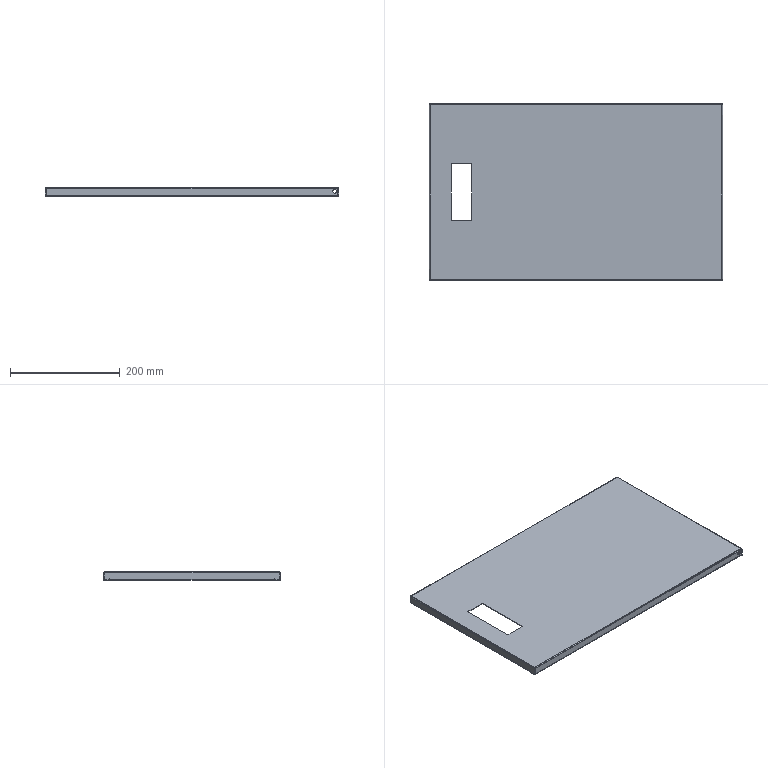Part | STEP file | 1 solid | 102 faces | box 533 x 321 x 15 mm | volume 244434 mm3 | plane 74 | cylinder 20 | spline 8 | commonest cylinder face diameters 1 x8 3.4 x8 7 x4